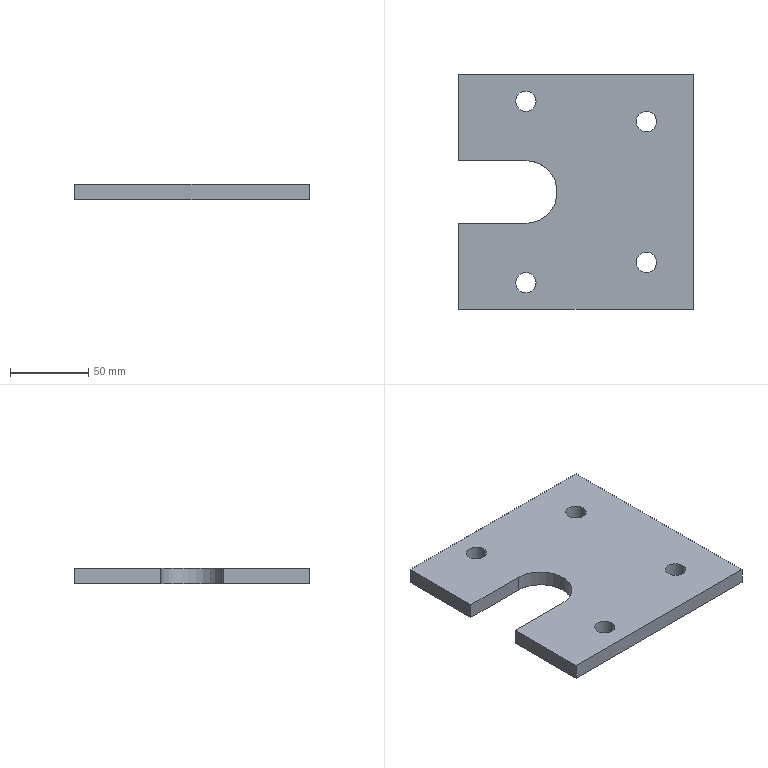Part | SolidWorks | features BaseBody 1 | 1 solid | 18 faces | box 150 x 150 x 10 mm | volume 196208 mm3 | cylinder 9 | plane 9 | commonest cylinder face diameters 13 x8 40 x1
STEP:
#1=CARTESIAN_POINT('',(-100.5,133.,0.));
#2=VERTEX_POINT('',#1);
#3=CARTESIAN_POINT('',(-113.5,133.,0.));
#4=VERTEX_POINT('',#3);
#5=CARTESIAN_POINT('',(-107.,133.,0.));
#6=DIRECTION('',(0.,0.,-1.));
#7=DIRECTION('',(1.,0.,0.));
#8=AXIS2_PLACEMENT_3D('',#5,#6,#7);
#9=CIRCLE('',#8,6.5);
#10=EDGE_CURVE('',#2,#4,#9,.T.);
#11=ORIENTED_EDGE('',*,*,#10,.T.);
#12=CARTESIAN_POINT('',(-113.5,133.,10.));
#13=VERTEX_POINT('',#12);
#14=CARTESIAN_POINT('',(-113.5,133.,-202.368));
#15=DIRECTION('',(0.,0.,1.));
#16=VECTOR('',#15,1000.);
#17=LINE('',#14,#16);
#18=EDGE_CURVE('',#4,#13,#17,.T.);
#19=ORIENTED_EDGE('',*,*,#18,.T.);
#20=CARTESIAN_POINT('',(-100.5,133.,10.));
#21=VERTEX_POINT('',#20);
#22=CARTESIAN_POINT('',(-107.,133.,10.));
#23=DIRECTION('',(0.,0.,-1.));
#24=DIRECTION('',(1.,0.,0.));
#25=AXIS2_PLACEMENT_3D('',#22,#23,#24);
#26=CIRCLE('',#25,6.5);
#27=EDGE_CURVE('',#21,#13,#26,.T.);
#28=ORIENTED_EDGE('',*,*,#27,.F.);
#29=CARTESIAN_POINT('',(-100.5,133.,-202.368));
#30=DIRECTION('',(0.,0.,1.));
#31=VECTOR('',#30,1000.);
#32=LINE('',#29,#31);
#33=EDGE_CURVE('',#2,#21,#32,.T.);
#34=ORIENTED_EDGE('',*,*,#33,.F.);
#35=EDGE_LOOP('',(#11,#19,#28,#34));
#36=FACE_OUTER_BOUND('',#35,.T.);
#37=CARTESIAN_POINT('',(-107.,133.,-202.368));
#38=DIRECTION('',(0.,0.,1.));
#39=DIRECTION('',(1.,0.,0.));
#40=AXIS2_PLACEMENT_3D('',#37,#38,#39);
#41=CYLINDRICAL_SURFACE('',#40,6.5);
#42=ADVANCED_FACE('',(#36),#41,.F.);
#43=CARTESIAN_POINT('',(-100.5,17.,0.));
#44=VERTEX_POINT('',#43);
#45=CARTESIAN_POINT('',(-113.5,17.,0.));
#46=VERTEX_POINT('',#45);
#47=CARTESIAN_POINT('',(-107.,17.,0.));
#48=DIRECTION('',(0.,0.,-1.));
#49=DIRECTION('',(1.,0.,0.));
#50=AXIS2_PLACEMENT_3D('',#47,#48,#49);
#51=CIRCLE('',#50,6.5);
#52=EDGE_CURVE('',#44,#46,#51,.T.);
#53=ORIENTED_EDGE('',*,*,#52,.T.);
#54=CARTESIAN_POINT('',(-113.5,17.,10.));
#55=VERTEX_POINT('',#54);
#56=CARTESIAN_POINT('',(-113.5,17.,-202.368));
#57=DIRECTION('',(0.,0.,1.));
#58=VECTOR('',#57,1000.);
#59=LINE('',#56,#58);
#60=EDGE_CURVE('',#46,#55,#59,.T.);
#61=ORIENTED_EDGE('',*,*,#60,.T.);
#62=CARTESIAN_POINT('',(-100.5,17.,10.));
#63=VERTEX_POINT('',#62);
#64=CARTESIAN_POINT('',(-107.,17.,10.));
#65=DIRECTION('',(0.,0.,-1.));
#66=DIRECTION('',(1.,0.,0.));
#67=AXIS2_PLACEMENT_3D('',#64,#65,#66);
#68=CIRCLE('',#67,6.5);
#69=EDGE_CURVE('',#63,#55,#68,.T.);
#70=ORIENTED_EDGE('',*,*,#69,.F.);
#71=CARTESIAN_POINT('',(-100.5,17.,-202.368));
#72=DIRECTION('',(0.,0.,1.));
#73=VECTOR('',#72,1000.);
#74=LINE('',#71,#73);
#75=EDGE_CURVE('',#44,#63,#74,.T.);
#76=ORIENTED_EDGE('',*,*,#75,.F.);
#77=EDGE_LOOP('',(#53,#61,#70,#76));
#78=FACE_OUTER_BOUND('',#77,.T.);
#79=CARTESIAN_POINT('',(-107.,17.,-202.368));
#80=DIRECTION('',(0.,0.,1.));
#81=DIRECTION('',(1.,0.,0.));
#82=AXIS2_PLACEMENT_3D('',#79,#80,#81);
#83=CYLINDRICAL_SURFACE('',#82,6.5);
#84=ADVANCED_FACE('',(#78),#83,.F.);
#85=CARTESIAN_POINT('',(-23.5,30.,10.));
#86=VERTEX_POINT('',#85);
#87=CARTESIAN_POINT('',(-36.5,30.,10.));
#88=VERTEX_POINT('',#87);
#89=CARTESIAN_POINT('',(-30.,30.,10.));
#90=DIRECTION('',(0.,0.,-1.));
#91=DIRECTION('',(-1.,0.,0.));
#92=AXIS2_PLACEMENT_3D('',#89,#90,#91);
#93=CIRCLE('',#92,6.5);
#94=EDGE_CURVE('',#86,#88,#93,.T.);
#95=ORIENTED_EDGE('',*,*,#94,.F.);
#96=CARTESIAN_POINT('',(-23.5,30.,0.));
#97=VERTEX_POINT('',#96);
#98=CARTESIAN_POINT('',(-23.5,30.,10.));
#99=DIRECTION('',(0.,0.,-1.));
#100=VECTOR('',#99,1000.);
#101=LINE('',#98,#100);
#102=EDGE_CURVE('',#86,#97,#101,.T.);
#103=ORIENTED_EDGE('',*,*,#102,.T.);
#104=CARTESIAN_POINT('',(-36.5,30.,0.));
#105=VERTEX_POINT('',#104);
#106=CARTESIAN_POINT('',(-30.,30.,0.));
#107=DIRECTION('',(0.,0.,-1.));
#108=DIRECTION('',(-1.,0.,0.));
#109=AXIS2_PLACEMENT_3D('',#106,#107,#108);
#110=CIRCLE('',#109,6.5);
#111=EDGE_CURVE('',#97,#105,#110,.T.);
#112=ORIENTED_EDGE('',*,*,#111,.T.);
#113=CARTESIAN_POINT('',(-36.5,30.,10.));
#114=DIRECTION('',(0.,0.,-1.));
#115=VECTOR('',#114,1000.);
#116=LINE('',#113,#115);
#117=EDGE_CURVE('',#88,#105,#116,.T.);
#118=ORIENTED_EDGE('',*,*,#117,.F.);
#119=EDGE_LOOP('',(#95,#103,#112,#118));
#120=FACE_OUTER_BOUND('',#119,.T.);
#121=CARTESIAN_POINT('',(-30.,30.,10.));
#122=DIRECTION('',(0.,0.,-1.));
#123=DIRECTION('',(-1.,0.,0.));
#124=AXIS2_PLACEMENT_3D('',#121,#122,#123);
#125=CYLINDRICAL_SURFACE('',#124,6.5);
#126=ADVANCED_FACE('',(#120),#125,.F.);
#127=CARTESIAN_POINT('',(-23.5,120.,10.));
#128=VERTEX_POINT('',#127);
#129=CARTESIAN_POINT('',(-36.5,120.,10.));
#130=VERTEX_POINT('',#129);
#131=CARTESIAN_POINT('',(-30.,120.,10.));
#132=DIRECTION('',(0.,0.,-1.));
#133=DIRECTION('',(-1.,0.,0.));
#134=AXIS2_PLACEMENT_3D('',#131,#132,#133);
#135=CIRCLE('',#134,6.5);
#136=EDGE_CURVE('',#128,#130,#135,.T.);
#137=ORIENTED_EDGE('',*,*,#136,.F.);
#138=CARTESIAN_POINT('',(-23.5,120.,0.));
#139=VERTEX_POINT('',#138);
#140=CARTESIAN_POINT('',(-23.5,120.,10.));
#141=DIRECTION('',(0.,0.,-1.));
#142=VECTOR('',#141,1000.);
#143=LINE('',#140,#142);
#144=EDGE_CURVE('',#128,#139,#143,.T.);
#145=ORIENTED_EDGE('',*,*,#144,.T.);
#146=CARTESIAN_POINT('',(-36.5,120.,0.));
#147=VERTEX_POINT('',#146);
#148=CARTESIAN_POINT('',(-30.,120.,0.));
#149=DIRECTION('',(0.,0.,-1.));
#150=DIRECTION('',(-1.,0.,0.));
#151=AXIS2_PLACEMENT_3D('',#148,#149,#150);
#152=CIRCLE('',#151,6.5);
#153=EDGE_CURVE('',#139,#147,#152,.T.);
#154=ORIENTED_EDGE('',*,*,#153,.T.);
#155=CARTESIAN_POINT('',(-36.5,120.,10.));
#156=DIRECTION('',(0.,0.,-1.));
#157=VECTOR('',#156,1000.);
#158=LINE('',#155,#157);
#159=EDGE_CURVE('',#130,#147,#158,.T.);
#160=ORIENTED_EDGE('',*,*,#159,.F.);
#161=EDGE_LOOP('',(#137,#145,#154,#160));
#162=FACE_OUTER_BOUND('',#161,.T.);
#163=CARTESIAN_POINT('',(-30.,120.,10.));
#164=DIRECTION('',(0.,0.,-1.));
#165=DIRECTION('',(-1.,0.,0.));
#166=AXIS2_PLACEMENT_3D('',#163,#164,#165);
#167=CYLINDRICAL_SURFACE('',#166,6.5);
#168=ADVANCED_FACE('',(#162),#167,.F.);
#169=ORIENTED_EDGE('',*,*,#10,.F.);
#170=CARTESIAN_POINT('',(-107.,133.,0.));
#171=DIRECTION('',(0.,0.,-1.));
#172=DIRECTION('',(1.,0.,0.));
#173=AXIS2_PLACEMENT_3D('',#170,#171,#172);
#174=CIRCLE('',#173,6.5);
#175=EDGE_CURVE('',#4,#2,#174,.T.);
#176=ORIENTED_EDGE('',*,*,#175,.F.);
#177=EDGE_LOOP('',(#169,#176));
#178=FACE_BOUND('',#177,.T.);
#179=ORIENTED_EDGE('',*,*,#52,.F.);
#180=CARTESIAN_POINT('',(-107.,17.,0.));
#181=DIRECTION('',(0.,0.,-1.));
#182=DIRECTION('',(1.,0.,0.));
#183=AXIS2_PLACEMENT_3D('',#180,#181,#182);
#184=CIRCLE('',#183,6.5);
#185=EDGE_CURVE('',#46,#44,#184,.T.);
#186=ORIENTED_EDGE('',*,*,#185,.F.);
#187=EDGE_LOOP('',(#179,#186));
#188=FACE_BOUND('',#187,.T.);
#189=CARTESIAN_POINT('',(-30.,30.,0.));
#190=DIRECTION('',(0.,0.,-1.));
#191=DIRECTION('',(-1.,0.,0.));
#192=AXIS2_PLACEMENT_3D('',#189,#190,#191);
#193=CIRCLE('',#192,6.5);
#194=EDGE_CURVE('',#105,#97,#193,.T.);
#195=ORIENTED_EDGE('',*,*,#194,.F.);
#196=ORIENTED_EDGE('',*,*,#111,.F.);
#197=EDGE_LOOP('',(#195,#196));
#198=FACE_BOUND('',#197,.T.);
#199=CARTESIAN_POINT('',(-30.,120.,0.));
#200=DIRECTION('',(0.,0.,-1.));
#201=DIRECTION('',(-1.,0.,0.));
#202=AXIS2_PLACEMENT_3D('',#199,#200,#201);
#203=CIRCLE('',#202,6.5);
#204=EDGE_CURVE('',#147,#139,#203,.T.);
#205=ORIENTED_EDGE('',*,*,#204,.F.);
#206=ORIENTED_EDGE('',*,*,#153,.F.);
#207=EDGE_LOOP('',(#205,#206));
#208=FACE_BOUND('',#207,.T.);
#209=CARTESIAN_POINT('',(-107.,95.,0.));
#210=VERTEX_POINT('',#209);
#211=CARTESIAN_POINT('',(-107.,55.,0.));
#212=VERTEX_POINT('',#211);
#213=CARTESIAN_POINT('',(-107.,75.,0.));
#214=DIRECTION('',(0.,0.,-1.));
#215=DIRECTION('',(-1.,0.,0.));
#216=AXIS2_PLACEMENT_3D('',#213,#214,#215);
#217=CIRCLE('',#216,20.);
#218=EDGE_CURVE('',#210,#212,#217,.T.);
#219=ORIENTED_EDGE('',*,*,#218,.F.);
#220=CARTESIAN_POINT('',(-150.,95.,0.));
#221=VERTEX_POINT('',#220);
#222=CARTESIAN_POINT('',(-75.,95.,0.));
#223=DIRECTION('',(1.,0.,0.));
#224=VECTOR('',#223,1000.);
#225=LINE('',#222,#224);
#226=EDGE_CURVE('',#221,#210,#225,.T.);
#227=ORIENTED_EDGE('',*,*,#226,.F.);
#228=CARTESIAN_POINT('',(-150.,150.,0.));
#229=VERTEX_POINT('',#228);
#230=CARTESIAN_POINT('',(-150.,75.,0.));
#231=DIRECTION('',(0.,-1.,0.));
#232=VECTOR('',#231,1000.);
#233=LINE('',#230,#232);
#234=EDGE_CURVE('',#229,#221,#233,.T.);
#235=ORIENTED_EDGE('',*,*,#234,.F.);
#236=CARTESIAN_POINT('',(0.,150.,0.));
#237=VERTEX_POINT('',#236);
#238=CARTESIAN_POINT('',(-75.,150.,0.));
#239=DIRECTION('',(-1.,0.,0.));
#240=VECTOR('',#239,1000.);
#241=LINE('',#238,#240);
#242=EDGE_CURVE('',#237,#229,#241,.T.);
#243=ORIENTED_EDGE('',*,*,#242,.F.);
#244=CARTESIAN_POINT('',(0.,0.,0.));
#245=VERTEX_POINT('',#244);
#246=CARTESIAN_POINT('',(0.,75.,0.));
#247=DIRECTION('',(0.,1.,0.));
#248=VECTOR('',#247,1000.);
#249=LINE('',#246,#248);
#250=EDGE_CURVE('',#245,#237,#249,.T.);
#251=ORIENTED_EDGE('',*,*,#250,.F.);
#252=CARTESIAN_POINT('',(-150.,0.,0.));
#253=VERTEX_POINT('',#252);
#254=CARTESIAN_POINT('',(-75.,0.,0.));
#255=DIRECTION('',(1.,0.,0.));
#256=VECTOR('',#255,1000.);
#257=LINE('',#254,#256);
#258=EDGE_CURVE('',#253,#245,#257,.T.);
#259=ORIENTED_EDGE('',*,*,#258,.F.);
#260=CARTESIAN_POINT('',(-150.,55.,0.));
#261=VERTEX_POINT('',#260);
#262=CARTESIAN_POINT('',(-150.,75.,0.));
#263=DIRECTION('',(0.,-1.,0.));
#264=VECTOR('',#263,1000.);
#265=LINE('',#262,#264);
#266=EDGE_CURVE('',#261,#253,#265,.T.);
#267=ORIENTED_EDGE('',*,*,#266,.F.);
#268=CARTESIAN_POINT('',(-75.,55.,0.));
#269=DIRECTION('',(-1.,0.,0.));
#270=VECTOR('',#269,1000.);
#271=LINE('',#268,#270);
#272=EDGE_CURVE('',#212,#261,#271,.T.);
#273=ORIENTED_EDGE('',*,*,#272,.F.);
#274=EDGE_LOOP('',(#219,#227,#235,#243,#251,#259,#267,#273));
#275=FACE_OUTER_BOUND('',#274,.T.);
#276=CARTESIAN_POINT('',(-75.,75.,0.));
#277=DIRECTION('',(0.,0.,1.));
#278=DIRECTION('',(1.,0.,0.));
#279=AXIS2_PLACEMENT_3D('',#276,#277,#278);
#280=PLANE('',#279);
#281=ADVANCED_FACE('',(#178,#188,#198,#208,#275),#280,.F.);
#282=ORIENTED_EDGE('',*,*,#18,.F.);
#283=ORIENTED_EDGE('',*,*,#175,.T.);
#284=ORIENTED_EDGE('',*,*,#33,.T.);
#285=CARTESIAN_POINT('',(-107.,133.,10.));
#286=DIRECTION('',(0.,0.,-1.));
#287=DIRECTION('',(1.,0.,0.));
#288=AXIS2_PLACEMENT_3D('',#285,#286,#287);
#289=CIRCLE('',#288,6.5);
#290=EDGE_CURVE('',#13,#21,#289,.T.);
#291=ORIENTED_EDGE('',*,*,#290,.F.);
#292=EDGE_LOOP('',(#282,#283,#284,#291));
#293=FACE_OUTER_BOUND('',#292,.T.);
#294=CARTESIAN_POINT('',(-107.,133.,-202.368));
#295=DIRECTION('',(0.,0.,1.));
#296=DIRECTION('',(1.,0.,0.));
#297=AXIS2_PLACEMENT_3D('',#294,#295,#296);
#298=CYLINDRICAL_SURFACE('',#297,6.5);
#299=ADVANCED_FACE('',(#293),#298,.F.);
#300=ORIENTED_EDGE('',*,*,#60,.F.);
#301=ORIENTED_EDGE('',*,*,#185,.T.);
#302=ORIENTED_EDGE('',*,*,#75,.T.);
#303=CARTESIAN_POINT('',(-107.,17.,10.));
#304=DIRECTION('',(0.,0.,-1.));
#305=DIRECTION('',(1.,0.,0.));
#306=AXIS2_PLACEMENT_3D('',#303,#304,#305);
#307=CIRCLE('',#306,6.5);
#308=EDGE_CURVE('',#55,#63,#307,.T.);
#309=ORIENTED_EDGE('',*,*,#308,.F.);
#310=EDGE_LOOP('',(#300,#301,#302,#309));
#311=FACE_OUTER_BOUND('',#310,.T.);
#312=CARTESIAN_POINT('',(-107.,17.,-202.368));
#313=DIRECTION('',(0.,0.,1.));
#314=DIRECTION('',(1.,0.,0.));
#315=AXIS2_PLACEMENT_3D('',#312,#313,#314);
#316=CYLINDRICAL_SURFACE('',#315,6.5);
#317=ADVANCED_FACE('',(#311),#316,.F.);
#318=ORIENTED_EDGE('',*,*,#102,.F.);
#319=CARTESIAN_POINT('',(-30.,30.,10.));
#320=DIRECTION('',(0.,0.,-1.));
#321=DIRECTION('',(-1.,0.,0.));
#322=AXIS2_PLACEMENT_3D('',#319,#320,#321);
#323=CIRCLE('',#322,6.5);
#324=EDGE_CURVE('',#88,#86,#323,.T.);
#325=ORIENTED_EDGE('',*,*,#324,.F.);
#326=ORIENTED_EDGE('',*,*,#117,.T.);
#327=ORIENTED_EDGE('',*,*,#194,.T.);
#328=EDGE_LOOP('',(#318,#325,#326,#327));
#329=FACE_OUTER_BOUND('',#328,.T.);
#330=CARTESIAN_POINT('',(-30.,30.,10.));
#331=DIRECTION('',(0.,0.,-1.));
#332=DIRECTION('',(-1.,0.,0.));
#333=AXIS2_PLACEMENT_3D('',#330,#331,#332);
#334=CYLINDRICAL_SURFACE('',#333,6.5);
#335=ADVANCED_FACE('',(#329),#334,.F.);
#336=ORIENTED_EDGE('',*,*,#144,.F.);
#337=CARTESIAN_POINT('',(-30.,120.,10.));
#338=DIRECTION('',(0.,0.,-1.));
#339=DIRECTION('',(-1.,0.,0.));
#340=AXIS2_PLACEMENT_3D('',#337,#338,#339);
#341=CIRCLE('',#340,6.5);
#342=EDGE_CURVE('',#130,#128,#341,.T.);
#343=ORIENTED_EDGE('',*,*,#342,.F.);
#344=ORIENTED_EDGE('',*,*,#159,.T.);
#345=ORIENTED_EDGE('',*,*,#204,.T.);
#346=EDGE_LOOP('',(#336,#343,#344,#345));
#347=FACE_OUTER_BOUND('',#346,.T.);
#348=CARTESIAN_POINT('',(-30.,120.,10.));
#349=DIRECTION('',(0.,0.,-1.));
#350=DIRECTION('',(-1.,0.,0.));
#351=AXIS2_PLACEMENT_3D('',#348,#349,#350);
#352=CYLINDRICAL_SURFACE('',#351,6.5);
#353=ADVANCED_FACE('',(#347),#352,.F.);
#354=CARTESIAN_POINT('',(-107.,55.,10.));
#355=VERTEX_POINT('',#354);
#356=CARTESIAN_POINT('',(-107.,55.,10.));
#357=DIRECTION('',(0.,0.,1.));
#358=VECTOR('',#357,1000.);
#359=LINE('',#356,#358);
#360=EDGE_CURVE('',#212,#355,#359,.T.);
#361=ORIENTED_EDGE('',*,*,#360,.F.);
#362=ORIENTED_EDGE('',*,*,#272,.T.);
#363=CARTESIAN_POINT('',(-150.,55.,10.));
#364=VERTEX_POINT('',#363);
#365=CARTESIAN_POINT('',(-150.,55.,10.));
#366=DIRECTION('',(0.,0.,-1.));
#367=VECTOR('',#366,1000.);
#368=LINE('',#365,#367);
#369=EDGE_CURVE('',#364,#261,#368,.T.);
#370=ORIENTED_EDGE('',*,*,#369,.F.);
#371=CARTESIAN_POINT('',(-107.,55.,10.));
#372=DIRECTION('',(-1.,0.,0.));
#373=VECTOR('',#372,1000.);
#374=LINE('',#371,#373);
#375=EDGE_CURVE('',#355,#364,#374,.T.);
#376=ORIENTED_EDGE('',*,*,#375,.F.);
#377=EDGE_LOOP('',(#361,#362,#370,#376));
#378=FACE_OUTER_BOUND('',#377,.T.);
#379=CARTESIAN_POINT('',(-107.,55.,10.));
#380=DIRECTION('',(0.,-1.,0.));
#381=DIRECTION('',(1.,0.,0.));
#382=AXIS2_PLACEMENT_3D('',#379,#380,#381);
#383=PLANE('',#382);
#384=ADVANCED_FACE('',(#378),#383,.F.);
#385=CARTESIAN_POINT('',(-107.,95.,10.));
#386=VERTEX_POINT('',#385);
#387=CARTESIAN_POINT('',(-107.,95.,10.));
#388=DIRECTION('',(0.,0.,1.));
#389=VECTOR('',#388,1000.);
#390=LINE('',#387,#389);
#391=EDGE_CURVE('',#210,#386,#390,.T.);
#392=ORIENTED_EDGE('',*,*,#391,.F.);
#393=ORIENTED_EDGE('',*,*,#218,.T.);
#394=ORIENTED_EDGE('',*,*,#360,.T.);
#395=CARTESIAN_POINT('',(-107.,75.,10.));
#396=DIRECTION('',(0.,0.,-1.));
#397=DIRECTION('',(-1.,0.,0.));
#398=AXIS2_PLACEMENT_3D('',#395,#396,#397);
#399=CIRCLE('',#398,20.);
#400=EDGE_CURVE('',#386,#355,#399,.T.);
#401=ORIENTED_EDGE('',*,*,#400,.F.);
#402=EDGE_LOOP('',(#392,#393,#394,#401));
#403=FACE_OUTER_BOUND('',#402,.T.);
#404=CARTESIAN_POINT('',(-107.,75.,10.));
#405=DIRECTION('',(0.,0.,-1.));
#406=DIRECTION('',(-1.,0.,0.));
#407=AXIS2_PLACEMENT_3D('',#404,#405,#406);
#408=CYLINDRICAL_SURFACE('',#407,20.);
#409=ADVANCED_FACE('',(#403),#408,.F.);
#410=CARTESIAN_POINT('',(-150.,95.,10.));
#411=VERTEX_POINT('',#410);
#412=CARTESIAN_POINT('',(-150.,95.,10.));
#413=DIRECTION('',(0.,0.,1.));
#414=VECTOR('',#413,1000.);
#415=LINE('',#412,#414);
#416=EDGE_CURVE('',#221,#411,#415,.T.);
#417=ORIENTED_EDGE('',*,*,#416,.F.);
#418=ORIENTED_EDGE('',*,*,#226,.T.);
#419=ORIENTED_EDGE('',*,*,#391,.T.);
#420=CARTESIAN_POINT('',(-150.,95.,10.));
#421=DIRECTION('',(1.,0.,0.));
#422=VECTOR('',#421,1000.);
#423=LINE('',#420,#422);
#424=EDGE_CURVE('',#411,#386,#423,.T.);
#425=ORIENTED_EDGE('',*,*,#424,.F.);
#426=EDGE_LOOP('',(#417,#418,#419,#425));
#427=FACE_OUTER_BOUND('',#426,.T.);
#428=CARTESIAN_POINT('',(-150.,95.,10.));
#429=DIRECTION('',(0.,1.,0.));
#430=DIRECTION('',(0.,0.,1.));
#431=AXIS2_PLACEMENT_3D('',#428,#429,#430);
#432=PLANE('',#431);
#433=ADVANCED_FACE('',(#427),#432,.F.);
#434=CARTESIAN_POINT('',(-150.,150.,10.));
#435=VERTEX_POINT('',#434);
#436=CARTESIAN_POINT('',(-150.,150.,0.));
#437=DIRECTION('',(0.,0.,-1.));
#438=VECTOR('',#437,1000.);
#439=LINE('',#436,#438);
#440=EDGE_CURVE('',#435,#229,#439,.T.);
#441=ORIENTED_EDGE('',*,*,#440,.T.);
#442=ORIENTED_EDGE('',*,*,#234,.T.);
#443=ORIENTED_EDGE('',*,*,#416,.T.);
#444=CARTESIAN_POINT('',(-150.,0.,10.));
#445=DIRECTION('',(0.,1.,0.));
#446=VECTOR('',#445,1000.);
#447=LINE('',#444,#446);
#448=EDGE_CURVE('',#411,#435,#447,.T.);
#449=ORIENTED_EDGE('',*,*,#448,.T.);
#450=EDGE_LOOP('',(#441,#442,#443,#449));
#451=FACE_OUTER_BOUND('',#450,.T.);
#452=CARTESIAN_POINT('',(-150.,0.,0.));
#453=DIRECTION('',(-1.,0.,0.));
#454=DIRECTION('',(0.,-1.,0.));
#455=AXIS2_PLACEMENT_3D('',#452,#453,#454);
#456=PLANE('',#455);
#457=ADVANCED_FACE('',(#451),#456,.T.);
#458=ORIENTED_EDGE('',*,*,#242,.T.);
#459=ORIENTED_EDGE('',*,*,#440,.F.);
#460=CARTESIAN_POINT('',(0.,150.,10.));
#461=VERTEX_POINT('',#460);
#462=CARTESIAN_POINT('',(-150.,150.,10.));
#463=DIRECTION('',(1.,0.,0.));
#464=VECTOR('',#463,1000.);
#465=LINE('',#462,#464);
#466=EDGE_CURVE('',#435,#461,#465,.T.);
#467=ORIENTED_EDGE('',*,*,#466,.T.);
#468=CARTESIAN_POINT('',(0.,150.,0.));
#469=DIRECTION('',(0.,0.,-1.));
#470=VECTOR('',#469,1000.);
#471=LINE('',#468,#470);
#472=EDGE_CURVE('',#461,#237,#471,.T.);
#473=ORIENTED_EDGE('',*,*,#472,.T.);
#474=EDGE_LOOP('',(#458,#459,#467,#473));
#475=FACE_OUTER_BOUND('',#474,.T.);
#476=CARTESIAN_POINT('',(-150.,150.,0.));
#477=DIRECTION('',(0.,1.,0.));
#478=DIRECTION('',(-1.,0.,0.));
#479=AXIS2_PLACEMENT_3D('',#476,#477,#478);
#480=PLANE('',#479);
#481=ADVANCED_FACE('',(#475),#480,.T.);
#482=ORIENTED_EDGE('',*,*,#250,.T.);
#483=ORIENTED_EDGE('',*,*,#472,.F.);
#484=CARTESIAN_POINT('',(0.,0.,10.));
#485=VERTEX_POINT('',#484);
#486=CARTESIAN_POINT('',(0.,150.,10.));
#487=DIRECTION('',(0.,-1.,0.));
#488=VECTOR('',#487,1000.);
#489=LINE('',#486,#488);
#490=EDGE_CURVE('',#461,#485,#489,.T.);
#491=ORIENTED_EDGE('',*,*,#490,.T.);
#492=CARTESIAN_POINT('',(0.,0.,0.));
#493=DIRECTION('',(0.,0.,-1.));
#494=VECTOR('',#493,1000.);
#495=LINE('',#492,#494);
#496=EDGE_CURVE('',#485,#245,#495,.T.);
#497=ORIENTED_EDGE('',*,*,#496,.T.);
#498=EDGE_LOOP('',(#482,#483,#491,#497));
#499=FACE_OUTER_BOUND('',#498,.T.);
#500=CARTESIAN_POINT('',(0.,150.,0.));
#501=DIRECTION('',(1.,0.,0.));
#502=DIRECTION('',(0.,1.,0.));
#503=AXIS2_PLACEMENT_3D('',#500,#501,#502);
#504=PLANE('',#503);
#505=ADVANCED_FACE('',(#499),#504,.T.);
#506=ORIENTED_EDGE('',*,*,#258,.T.);
#507=ORIENTED_EDGE('',*,*,#496,.F.);
#508=CARTESIAN_POINT('',(-150.,0.,10.));
#509=VERTEX_POINT('',#508);
#510=CARTESIAN_POINT('',(0.,0.,10.));
#511=DIRECTION('',(-1.,0.,0.));
#512=VECTOR('',#511,1000.);
#513=LINE('',#510,#512);
#514=EDGE_CURVE('',#485,#509,#513,.T.);
#515=ORIENTED_EDGE('',*,*,#514,.T.);
#516=CARTESIAN_POINT('',(-150.,0.,0.));
#517=DIRECTION('',(0.,0.,-1.));
#518=VECTOR('',#517,1000.);
#519=LINE('',#516,#518);
#520=EDGE_CURVE('',#509,#253,#519,.T.);
#521=ORIENTED_EDGE('',*,*,#520,.T.);
#522=EDGE_LOOP('',(#506,#507,#515,#521));
#523=FACE_OUTER_BOUND('',#522,.T.);
#524=CARTESIAN_POINT('',(0.,0.,0.));
#525=DIRECTION('',(0.,-1.,0.));
#526=DIRECTION('',(1.,0.,0.));
#527=AXIS2_PLACEMENT_3D('',#524,#525,#526);
#528=PLANE('',#527);
#529=ADVANCED_FACE('',(#523),#528,.T.);
#530=ORIENTED_EDGE('',*,*,#520,.F.);
#531=CARTESIAN_POINT('',(-150.,0.,10.));
#532=DIRECTION('',(0.,1.,0.));
#533=VECTOR('',#532,1000.);
#534=LINE('',#531,#533);
#535=EDGE_CURVE('',#509,#364,#534,.T.);
#536=ORIENTED_EDGE('',*,*,#535,.T.);
#537=ORIENTED_EDGE('',*,*,#369,.T.);
#538=ORIENTED_EDGE('',*,*,#266,.T.);
#539=EDGE_LOOP('',(#530,#536,#537,#538));
#540=FACE_OUTER_BOUND('',#539,.T.);
#541=CARTESIAN_POINT('',(-150.,0.,0.));
#542=DIRECTION('',(-1.,0.,0.));
#543=DIRECTION('',(0.,-1.,0.));
#544=AXIS2_PLACEMENT_3D('',#541,#542,#543);
#545=PLANE('',#544);
#546=ADVANCED_FACE('',(#540),#545,.T.);
#547=ORIENTED_EDGE('',*,*,#69,.T.);
#548=ORIENTED_EDGE('',*,*,#308,.T.);
#549=EDGE_LOOP('',(#547,#548));
#550=FACE_BOUND('',#549,.T.);
#551=ORIENTED_EDGE('',*,*,#27,.T.);
#552=ORIENTED_EDGE('',*,*,#290,.T.);
#553=EDGE_LOOP('',(#551,#552));
#554=FACE_BOUND('',#553,.T.);
#555=ORIENTED_EDGE('',*,*,#324,.T.);
#556=ORIENTED_EDGE('',*,*,#94,.T.);
#557=EDGE_LOOP('',(#555,#556));
#558=FACE_BOUND('',#557,.T.);
#559=ORIENTED_EDGE('',*,*,#342,.T.);
#560=ORIENTED_EDGE('',*,*,#136,.T.);
#561=EDGE_LOOP('',(#559,#560));
#562=FACE_BOUND('',#561,.T.);
#563=ORIENTED_EDGE('',*,*,#424,.T.);
#564=ORIENTED_EDGE('',*,*,#400,.T.);
#565=ORIENTED_EDGE('',*,*,#375,.T.);
#566=ORIENTED_EDGE('',*,*,#535,.F.);
#567=ORIENTED_EDGE('',*,*,#514,.F.);
#568=ORIENTED_EDGE('',*,*,#490,.F.);
#569=ORIENTED_EDGE('',*,*,#466,.F.);
#570=ORIENTED_EDGE('',*,*,#448,.F.);
#571=EDGE_LOOP('',(#563,#564,#565,#566,#567,#568,#569,#570));
#572=FACE_OUTER_BOUND('',#571,.T.);
#573=CARTESIAN_POINT('',(-75.,75.,10.));
#574=DIRECTION('',(0.,0.,1.));
#575=DIRECTION('',(1.,0.,0.));
#576=AXIS2_PLACEMENT_3D('',#573,#574,#575);
#577=PLANE('',#576);
#578=ADVANCED_FACE('',(#550,#554,#558,#562,#572),#577,.T.);
#579=CLOSED_SHELL('',(#42,#84,#126,#168,#281,#299,#317,#335,#353,#384,#409,#433,#457,#481,#505,#529,#546,#578));
#580=MANIFOLD_SOLID_BREP('',#579);
#581=CARTESIAN_POINT('',(0.,0.,0.));
#582=DIRECTION('',(0.,0.,1.));
#583=DIRECTION('',(1.,0.,0.));
#584=AXIS2_PLACEMENT_3D('',#581,#582,#583);
#585=(LENGTH_UNIT()NAMED_UNIT(*)SI_UNIT(.MILLI.,.METRE.));
#586=UNCERTAINTY_MEASURE_WITH_UNIT(LENGTH_MEASURE(0.00001),#585,'','');
#587=(NAMED_UNIT(*)PLANE_ANGLE_UNIT()SI_UNIT($,.RADIAN.));
#588=(NAMED_UNIT(*)SI_UNIT($,.STERADIAN.)SOLID_ANGLE_UNIT());
#589=(GEOMETRIC_REPRESENTATION_CONTEXT(3)GLOBAL_UNCERTAINTY_ASSIGNED_CONTEXT((#586))GLOBAL_UNIT_ASSIGNED_CONTEXT((#585,#587,#588))REPRESENTATION_CONTEXT('',''));
#590=ADVANCED_BREP_SHAPE_REPRESENTATION('',(#580,#584),#589);